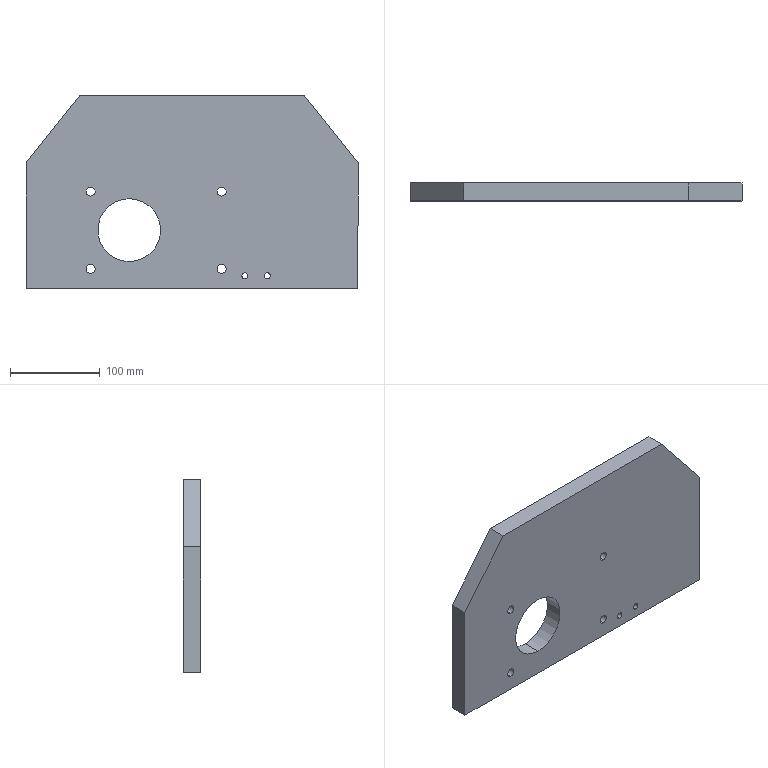Part | SolidWorks | features BaseBody 1 | 1 solid | 22 faces | box 370 x 20 x 215 mm | volume 1416295 mm3 | cylinder 14 | plane 8 | commonest cylinder face diameters 10 x8 6.8 x4 70 x2
STEP:
#1=CARTESIAN_POINT('',(-70.,0.,30.));
#2=VERTEX_POINT('',#1);
#3=CARTESIAN_POINT('',(-70.,0.,100.));
#4=VERTEX_POINT('',#3);
#5=CARTESIAN_POINT('',(-70.,0.,65.));
#6=DIRECTION('',(0.,1.,0.));
#7=DIRECTION('',(0.,0.,1.));
#8=AXIS2_PLACEMENT_3D('',#5,#6,#7);
#9=CIRCLE('',#8,35.);
#10=EDGE_CURVE('',#2,#4,#9,.T.);
#11=ORIENTED_EDGE('',*,*,#10,.F.);
#12=CARTESIAN_POINT('',(-70.,20.,30.));
#13=VERTEX_POINT('',#12);
#14=CARTESIAN_POINT('',(-70.,0.,30.));
#15=DIRECTION('',(0.,1.,0.));
#16=VECTOR('',#15,1000.);
#17=LINE('',#14,#16);
#18=EDGE_CURVE('',#2,#13,#17,.T.);
#19=ORIENTED_EDGE('',*,*,#18,.T.);
#20=CARTESIAN_POINT('',(-70.,20.,100.));
#21=VERTEX_POINT('',#20);
#22=CARTESIAN_POINT('',(-70.,20.,65.));
#23=DIRECTION('',(0.,-1.,0.));
#24=DIRECTION('',(0.,0.,1.));
#25=AXIS2_PLACEMENT_3D('',#22,#23,#24);
#26=CIRCLE('',#25,35.);
#27=EDGE_CURVE('',#21,#13,#26,.T.);
#28=ORIENTED_EDGE('',*,*,#27,.F.);
#29=CARTESIAN_POINT('',(-70.,0.,100.));
#30=DIRECTION('',(0.,1.,0.));
#31=VECTOR('',#30,1000.);
#32=LINE('',#29,#31);
#33=EDGE_CURVE('',#4,#21,#32,.T.);
#34=ORIENTED_EDGE('',*,*,#33,.F.);
#35=EDGE_LOOP('',(#11,#19,#28,#34));
#36=FACE_OUTER_BOUND('',#35,.T.);
#37=CARTESIAN_POINT('',(-70.,0.,65.));
#38=DIRECTION('',(0.,1.,0.));
#39=DIRECTION('',(0.,0.,1.));
#40=AXIS2_PLACEMENT_3D('',#37,#38,#39);
#41=CYLINDRICAL_SURFACE('',#40,35.);
#42=ADVANCED_FACE('',(#36),#41,.F.);
#43=CARTESIAN_POINT('',(-113.,0.,17.));
#44=VERTEX_POINT('',#43);
#45=CARTESIAN_POINT('',(-113.,0.,27.));
#46=VERTEX_POINT('',#45);
#47=CARTESIAN_POINT('',(-113.,0.,22.));
#48=DIRECTION('',(0.,1.,0.));
#49=DIRECTION('',(0.,0.,1.));
#50=AXIS2_PLACEMENT_3D('',#47,#48,#49);
#51=CIRCLE('',#50,5.);
#52=EDGE_CURVE('',#44,#46,#51,.T.);
#53=ORIENTED_EDGE('',*,*,#52,.F.);
#54=CARTESIAN_POINT('',(-113.,20.,17.));
#55=VERTEX_POINT('',#54);
#56=CARTESIAN_POINT('',(-113.,0.,17.));
#57=DIRECTION('',(0.,1.,0.));
#58=VECTOR('',#57,1000.);
#59=LINE('',#56,#58);
#60=EDGE_CURVE('',#44,#55,#59,.T.);
#61=ORIENTED_EDGE('',*,*,#60,.T.);
#62=CARTESIAN_POINT('',(-113.,20.,27.));
#63=VERTEX_POINT('',#62);
#64=CARTESIAN_POINT('',(-113.,20.,22.));
#65=DIRECTION('',(0.,-1.,0.));
#66=DIRECTION('',(0.,0.,1.));
#67=AXIS2_PLACEMENT_3D('',#64,#65,#66);
#68=CIRCLE('',#67,5.);
#69=EDGE_CURVE('',#63,#55,#68,.T.);
#70=ORIENTED_EDGE('',*,*,#69,.F.);
#71=CARTESIAN_POINT('',(-113.,0.,27.));
#72=DIRECTION('',(0.,1.,0.));
#73=VECTOR('',#72,1000.);
#74=LINE('',#71,#73);
#75=EDGE_CURVE('',#46,#63,#74,.T.);
#76=ORIENTED_EDGE('',*,*,#75,.F.);
#77=EDGE_LOOP('',(#53,#61,#70,#76));
#78=FACE_OUTER_BOUND('',#77,.T.);
#79=CARTESIAN_POINT('',(-113.,0.,22.));
#80=DIRECTION('',(0.,1.,0.));
#81=DIRECTION('',(0.,0.,1.));
#82=AXIS2_PLACEMENT_3D('',#79,#80,#81);
#83=CYLINDRICAL_SURFACE('',#82,5.);
#84=ADVANCED_FACE('',(#78),#83,.F.);
#85=CARTESIAN_POINT('',(33.,0.,17.));
#86=VERTEX_POINT('',#85);
#87=CARTESIAN_POINT('',(33.,0.,27.));
#88=VERTEX_POINT('',#87);
#89=CARTESIAN_POINT('',(33.,0.,22.));
#90=DIRECTION('',(0.,1.,0.));
#91=DIRECTION('',(0.,0.,1.));
#92=AXIS2_PLACEMENT_3D('',#89,#90,#91);
#93=CIRCLE('',#92,5.);
#94=EDGE_CURVE('',#86,#88,#93,.T.);
#95=ORIENTED_EDGE('',*,*,#94,.F.);
#96=CARTESIAN_POINT('',(33.,20.,17.));
#97=VERTEX_POINT('',#96);
#98=CARTESIAN_POINT('',(33.,0.,17.));
#99=DIRECTION('',(0.,1.,0.));
#100=VECTOR('',#99,1000.);
#101=LINE('',#98,#100);
#102=EDGE_CURVE('',#86,#97,#101,.T.);
#103=ORIENTED_EDGE('',*,*,#102,.T.);
#104=CARTESIAN_POINT('',(33.,20.,27.));
#105=VERTEX_POINT('',#104);
#106=CARTESIAN_POINT('',(33.,20.,22.));
#107=DIRECTION('',(0.,-1.,0.));
#108=DIRECTION('',(0.,0.,1.));
#109=AXIS2_PLACEMENT_3D('',#106,#107,#108);
#110=CIRCLE('',#109,5.);
#111=EDGE_CURVE('',#105,#97,#110,.T.);
#112=ORIENTED_EDGE('',*,*,#111,.F.);
#113=CARTESIAN_POINT('',(33.,0.,27.));
#114=DIRECTION('',(0.,1.,0.));
#115=VECTOR('',#114,1000.);
#116=LINE('',#113,#115);
#117=EDGE_CURVE('',#88,#105,#116,.T.);
#118=ORIENTED_EDGE('',*,*,#117,.F.);
#119=EDGE_LOOP('',(#95,#103,#112,#118));
#120=FACE_OUTER_BOUND('',#119,.T.);
#121=CARTESIAN_POINT('',(33.,0.,22.));
#122=DIRECTION('',(0.,1.,0.));
#123=DIRECTION('',(0.,0.,1.));
#124=AXIS2_PLACEMENT_3D('',#121,#122,#123);
#125=CYLINDRICAL_SURFACE('',#124,5.);
#126=ADVANCED_FACE('',(#120),#125,.F.);
#127=CARTESIAN_POINT('',(33.,0.,103.));
#128=VERTEX_POINT('',#127);
#129=CARTESIAN_POINT('',(33.,0.,113.));
#130=VERTEX_POINT('',#129);
#131=CARTESIAN_POINT('',(33.,0.,108.));
#132=DIRECTION('',(0.,1.,0.));
#133=DIRECTION('',(0.,0.,1.));
#134=AXIS2_PLACEMENT_3D('',#131,#132,#133);
#135=CIRCLE('',#134,5.);
#136=EDGE_CURVE('',#128,#130,#135,.T.);
#137=ORIENTED_EDGE('',*,*,#136,.F.);
#138=CARTESIAN_POINT('',(33.,20.,103.));
#139=VERTEX_POINT('',#138);
#140=CARTESIAN_POINT('',(33.,0.,103.));
#141=DIRECTION('',(0.,1.,0.));
#142=VECTOR('',#141,1000.);
#143=LINE('',#140,#142);
#144=EDGE_CURVE('',#128,#139,#143,.T.);
#145=ORIENTED_EDGE('',*,*,#144,.T.);
#146=CARTESIAN_POINT('',(33.,20.,113.));
#147=VERTEX_POINT('',#146);
#148=CARTESIAN_POINT('',(33.,20.,108.));
#149=DIRECTION('',(0.,-1.,0.));
#150=DIRECTION('',(0.,0.,1.));
#151=AXIS2_PLACEMENT_3D('',#148,#149,#150);
#152=CIRCLE('',#151,5.);
#153=EDGE_CURVE('',#147,#139,#152,.T.);
#154=ORIENTED_EDGE('',*,*,#153,.F.);
#155=CARTESIAN_POINT('',(33.,0.,113.));
#156=DIRECTION('',(0.,1.,0.));
#157=VECTOR('',#156,1000.);
#158=LINE('',#155,#157);
#159=EDGE_CURVE('',#130,#147,#158,.T.);
#160=ORIENTED_EDGE('',*,*,#159,.F.);
#161=EDGE_LOOP('',(#137,#145,#154,#160));
#162=FACE_OUTER_BOUND('',#161,.T.);
#163=CARTESIAN_POINT('',(33.,0.,108.));
#164=DIRECTION('',(0.,1.,0.));
#165=DIRECTION('',(0.,0.,1.));
#166=AXIS2_PLACEMENT_3D('',#163,#164,#165);
#167=CYLINDRICAL_SURFACE('',#166,5.);
#168=ADVANCED_FACE('',(#162),#167,.F.);
#169=CARTESIAN_POINT('',(-113.,0.,103.));
#170=VERTEX_POINT('',#169);
#171=CARTESIAN_POINT('',(-113.,0.,113.));
#172=VERTEX_POINT('',#171);
#173=CARTESIAN_POINT('',(-113.,0.,108.));
#174=DIRECTION('',(0.,1.,0.));
#175=DIRECTION('',(0.,0.,1.));
#176=AXIS2_PLACEMENT_3D('',#173,#174,#175);
#177=CIRCLE('',#176,5.);
#178=EDGE_CURVE('',#170,#172,#177,.T.);
#179=ORIENTED_EDGE('',*,*,#178,.F.);
#180=CARTESIAN_POINT('',(-113.,20.,103.));
#181=VERTEX_POINT('',#180);
#182=CARTESIAN_POINT('',(-113.,0.,103.));
#183=DIRECTION('',(0.,1.,0.));
#184=VECTOR('',#183,1000.);
#185=LINE('',#182,#184);
#186=EDGE_CURVE('',#170,#181,#185,.T.);
#187=ORIENTED_EDGE('',*,*,#186,.T.);
#188=CARTESIAN_POINT('',(-113.,20.,113.));
#189=VERTEX_POINT('',#188);
#190=CARTESIAN_POINT('',(-113.,20.,108.));
#191=DIRECTION('',(0.,-1.,0.));
#192=DIRECTION('',(0.,0.,1.));
#193=AXIS2_PLACEMENT_3D('',#190,#191,#192);
#194=CIRCLE('',#193,5.);
#195=EDGE_CURVE('',#189,#181,#194,.T.);
#196=ORIENTED_EDGE('',*,*,#195,.F.);
#197=CARTESIAN_POINT('',(-113.,0.,113.));
#198=DIRECTION('',(0.,1.,0.));
#199=VECTOR('',#198,1000.);
#200=LINE('',#197,#199);
#201=EDGE_CURVE('',#172,#189,#200,.T.);
#202=ORIENTED_EDGE('',*,*,#201,.F.);
#203=EDGE_LOOP('',(#179,#187,#196,#202));
#204=FACE_OUTER_BOUND('',#203,.T.);
#205=CARTESIAN_POINT('',(-113.,0.,108.));
#206=DIRECTION('',(0.,1.,0.));
#207=DIRECTION('',(0.,0.,1.));
#208=AXIS2_PLACEMENT_3D('',#205,#206,#207);
#209=CYLINDRICAL_SURFACE('',#208,5.);
#210=ADVANCED_FACE('',(#204),#209,.F.);
#211=CARTESIAN_POINT('',(83.921,20.,17.4));
#212=VERTEX_POINT('',#211);
#213=CARTESIAN_POINT('',(83.921,20.,10.6));
#214=VERTEX_POINT('',#213);
#215=CARTESIAN_POINT('',(83.921,20.,14.));
#216=DIRECTION('',(0.,-1.,0.));
#217=DIRECTION('',(0.,0.,-1.));
#218=AXIS2_PLACEMENT_3D('',#215,#216,#217);
#219=CIRCLE('',#218,3.4);
#220=EDGE_CURVE('',#212,#214,#219,.T.);
#221=ORIENTED_EDGE('',*,*,#220,.F.);
#222=CARTESIAN_POINT('',(83.921,0.,17.4));
#223=VERTEX_POINT('',#222);
#224=CARTESIAN_POINT('',(83.921,0.,17.4));
#225=DIRECTION('',(0.,-1.,0.));
#226=VECTOR('',#225,1000.);
#227=LINE('',#224,#226);
#228=EDGE_CURVE('',#212,#223,#227,.T.);
#229=ORIENTED_EDGE('',*,*,#228,.T.);
#230=CARTESIAN_POINT('',(83.921,0.,10.6));
#231=VERTEX_POINT('',#230);
#232=CARTESIAN_POINT('',(83.921,0.,14.));
#233=DIRECTION('',(0.,1.,0.));
#234=DIRECTION('',(0.,0.,-1.));
#235=AXIS2_PLACEMENT_3D('',#232,#233,#234);
#236=CIRCLE('',#235,3.4);
#237=EDGE_CURVE('',#231,#223,#236,.T.);
#238=ORIENTED_EDGE('',*,*,#237,.F.);
#239=CARTESIAN_POINT('',(83.921,0.,10.6));
#240=DIRECTION('',(0.,-1.,0.));
#241=VECTOR('',#240,1000.);
#242=LINE('',#239,#241);
#243=EDGE_CURVE('',#214,#231,#242,.T.);
#244=ORIENTED_EDGE('',*,*,#243,.F.);
#245=EDGE_LOOP('',(#221,#229,#238,#244));
#246=FACE_OUTER_BOUND('',#245,.T.);
#247=CARTESIAN_POINT('',(83.921,0.,14.));
#248=DIRECTION('',(0.,-1.,0.));
#249=DIRECTION('',(0.,0.,-1.));
#250=AXIS2_PLACEMENT_3D('',#247,#248,#249);
#251=CYLINDRICAL_SURFACE('',#250,3.4);
#252=ADVANCED_FACE('',(#246),#251,.F.);
#253=CARTESIAN_POINT('',(58.921,20.,17.4));
#254=VERTEX_POINT('',#253);
#255=CARTESIAN_POINT('',(58.921,20.,10.6));
#256=VERTEX_POINT('',#255);
#257=CARTESIAN_POINT('',(58.921,20.,14.));
#258=DIRECTION('',(0.,-1.,0.));
#259=DIRECTION('',(0.,0.,-1.));
#260=AXIS2_PLACEMENT_3D('',#257,#258,#259);
#261=CIRCLE('',#260,3.4);
#262=EDGE_CURVE('',#254,#256,#261,.T.);
#263=ORIENTED_EDGE('',*,*,#262,.F.);
#264=CARTESIAN_POINT('',(58.921,0.,17.4));
#265=VERTEX_POINT('',#264);
#266=CARTESIAN_POINT('',(58.921,0.,17.4));
#267=DIRECTION('',(0.,-1.,0.));
#268=VECTOR('',#267,1000.);
#269=LINE('',#266,#268);
#270=EDGE_CURVE('',#254,#265,#269,.T.);
#271=ORIENTED_EDGE('',*,*,#270,.T.);
#272=CARTESIAN_POINT('',(58.921,0.,10.6));
#273=VERTEX_POINT('',#272);
#274=CARTESIAN_POINT('',(58.921,0.,14.));
#275=DIRECTION('',(0.,1.,0.));
#276=DIRECTION('',(0.,0.,-1.));
#277=AXIS2_PLACEMENT_3D('',#274,#275,#276);
#278=CIRCLE('',#277,3.4);
#279=EDGE_CURVE('',#273,#265,#278,.T.);
#280=ORIENTED_EDGE('',*,*,#279,.F.);
#281=CARTESIAN_POINT('',(58.921,0.,10.6));
#282=DIRECTION('',(0.,-1.,0.));
#283=VECTOR('',#282,1000.);
#284=LINE('',#281,#283);
#285=EDGE_CURVE('',#256,#273,#284,.T.);
#286=ORIENTED_EDGE('',*,*,#285,.F.);
#287=EDGE_LOOP('',(#263,#271,#280,#286));
#288=FACE_OUTER_BOUND('',#287,.T.);
#289=CARTESIAN_POINT('',(58.921,0.,14.));
#290=DIRECTION('',(0.,-1.,0.));
#291=DIRECTION('',(0.,0.,-1.));
#292=AXIS2_PLACEMENT_3D('',#289,#290,#291);
#293=CYLINDRICAL_SURFACE('',#292,3.4);
#294=ADVANCED_FACE('',(#288),#293,.F.);
#295=CARTESIAN_POINT('',(185.,20.,140.));
#296=VERTEX_POINT('',#295);
#297=CARTESIAN_POINT('',(185.,20.,0.));
#298=VERTEX_POINT('',#297);
#299=CARTESIAN_POINT('',(185.,20.,0.));
#300=DIRECTION('',(0.,0.,-1.));
#301=VECTOR('',#300,1000.);
#302=LINE('',#299,#301);
#303=EDGE_CURVE('',#296,#298,#302,.T.);
#304=ORIENTED_EDGE('',*,*,#303,.T.);
#305=CARTESIAN_POINT('',(-185.,20.,0.));
#306=VERTEX_POINT('',#305);
#307=CARTESIAN_POINT('',(0.,20.,0.));
#308=DIRECTION('',(-1.,0.,0.));
#309=VECTOR('',#308,1000.);
#310=LINE('',#307,#309);
#311=EDGE_CURVE('',#298,#306,#310,.T.);
#312=ORIENTED_EDGE('',*,*,#311,.T.);
#313=CARTESIAN_POINT('',(-185.,20.,140.));
#314=VERTEX_POINT('',#313);
#315=CARTESIAN_POINT('',(-185.,20.,0.));
#316=DIRECTION('',(0.,0.,1.));
#317=VECTOR('',#316,1000.);
#318=LINE('',#315,#317);
#319=EDGE_CURVE('',#306,#314,#318,.T.);
#320=ORIENTED_EDGE('',*,*,#319,.T.);
#321=CARTESIAN_POINT('',(-125.,20.,215.));
#322=VERTEX_POINT('',#321);
#323=CARTESIAN_POINT('',(-185.,20.,140.));
#324=DIRECTION('',(0.6247,0.,0.7809));
#325=VECTOR('',#324,1000.);
#326=LINE('',#323,#325);
#327=EDGE_CURVE('',#314,#322,#326,.T.);
#328=ORIENTED_EDGE('',*,*,#327,.T.);
#329=CARTESIAN_POINT('',(125.,20.,215.));
#330=VERTEX_POINT('',#329);
#331=CARTESIAN_POINT('',(0.,20.,215.));
#332=DIRECTION('',(1.,0.,0.));
#333=VECTOR('',#332,1000.);
#334=LINE('',#331,#333);
#335=EDGE_CURVE('',#322,#330,#334,.T.);
#336=ORIENTED_EDGE('',*,*,#335,.T.);
#337=CARTESIAN_POINT('',(125.,20.,215.));
#338=DIRECTION('',(0.6247,0.,-0.7809));
#339=VECTOR('',#338,1000.);
#340=LINE('',#337,#339);
#341=EDGE_CURVE('',#330,#296,#340,.T.);
#342=ORIENTED_EDGE('',*,*,#341,.T.);
#343=EDGE_LOOP('',(#304,#312,#320,#328,#336,#342));
#344=FACE_OUTER_BOUND('',#343,.T.);
#345=ORIENTED_EDGE('',*,*,#27,.T.);
#346=CARTESIAN_POINT('',(-70.,20.,65.));
#347=DIRECTION('',(0.,-1.,0.));
#348=DIRECTION('',(0.,0.,1.));
#349=AXIS2_PLACEMENT_3D('',#346,#347,#348);
#350=CIRCLE('',#349,35.);
#351=EDGE_CURVE('',#13,#21,#350,.T.);
#352=ORIENTED_EDGE('',*,*,#351,.T.);
#353=EDGE_LOOP('',(#345,#352));
#354=FACE_BOUND('',#353,.T.);
#355=ORIENTED_EDGE('',*,*,#69,.T.);
#356=CARTESIAN_POINT('',(-113.,20.,22.));
#357=DIRECTION('',(0.,-1.,0.));
#358=DIRECTION('',(0.,0.,1.));
#359=AXIS2_PLACEMENT_3D('',#356,#357,#358);
#360=CIRCLE('',#359,5.);
#361=EDGE_CURVE('',#55,#63,#360,.T.);
#362=ORIENTED_EDGE('',*,*,#361,.T.);
#363=EDGE_LOOP('',(#355,#362));
#364=FACE_BOUND('',#363,.T.);
#365=ORIENTED_EDGE('',*,*,#111,.T.);
#366=CARTESIAN_POINT('',(33.,20.,22.));
#367=DIRECTION('',(0.,-1.,0.));
#368=DIRECTION('',(0.,0.,1.));
#369=AXIS2_PLACEMENT_3D('',#366,#367,#368);
#370=CIRCLE('',#369,5.);
#371=EDGE_CURVE('',#97,#105,#370,.T.);
#372=ORIENTED_EDGE('',*,*,#371,.T.);
#373=EDGE_LOOP('',(#365,#372));
#374=FACE_BOUND('',#373,.T.);
#375=ORIENTED_EDGE('',*,*,#153,.T.);
#376=CARTESIAN_POINT('',(33.,20.,108.));
#377=DIRECTION('',(0.,-1.,0.));
#378=DIRECTION('',(0.,0.,1.));
#379=AXIS2_PLACEMENT_3D('',#376,#377,#378);
#380=CIRCLE('',#379,5.);
#381=EDGE_CURVE('',#139,#147,#380,.T.);
#382=ORIENTED_EDGE('',*,*,#381,.T.);
#383=EDGE_LOOP('',(#375,#382));
#384=FACE_BOUND('',#383,.T.);
#385=ORIENTED_EDGE('',*,*,#195,.T.);
#386=CARTESIAN_POINT('',(-113.,20.,108.));
#387=DIRECTION('',(0.,-1.,0.));
#388=DIRECTION('',(0.,0.,1.));
#389=AXIS2_PLACEMENT_3D('',#386,#387,#388);
#390=CIRCLE('',#389,5.);
#391=EDGE_CURVE('',#181,#189,#390,.T.);
#392=ORIENTED_EDGE('',*,*,#391,.T.);
#393=EDGE_LOOP('',(#385,#392));
#394=FACE_BOUND('',#393,.T.);
#395=CARTESIAN_POINT('',(83.921,20.,14.));
#396=DIRECTION('',(0.,-1.,0.));
#397=DIRECTION('',(0.,0.,-1.));
#398=AXIS2_PLACEMENT_3D('',#395,#396,#397);
#399=CIRCLE('',#398,3.4);
#400=EDGE_CURVE('',#214,#212,#399,.T.);
#401=ORIENTED_EDGE('',*,*,#400,.T.);
#402=ORIENTED_EDGE('',*,*,#220,.T.);
#403=EDGE_LOOP('',(#401,#402));
#404=FACE_BOUND('',#403,.T.);
#405=CARTESIAN_POINT('',(58.921,20.,14.));
#406=DIRECTION('',(0.,-1.,0.));
#407=DIRECTION('',(0.,0.,-1.));
#408=AXIS2_PLACEMENT_3D('',#405,#406,#407);
#409=CIRCLE('',#408,3.4);
#410=EDGE_CURVE('',#256,#254,#409,.T.);
#411=ORIENTED_EDGE('',*,*,#410,.T.);
#412=ORIENTED_EDGE('',*,*,#262,.T.);
#413=EDGE_LOOP('',(#411,#412));
#414=FACE_BOUND('',#413,.T.);
#415=CARTESIAN_POINT('',(0.,20.,0.));
#416=DIRECTION('',(0.,1.,0.));
#417=DIRECTION('',(0.,0.,1.));
#418=AXIS2_PLACEMENT_3D('',#415,#416,#417);
#419=PLANE('',#418);
#420=ADVANCED_FACE('',(#344,#354,#364,#374,#384,#394,#404,#414),#419,.T.);
#421=CARTESIAN_POINT('',(-185.,0.,0.));
#422=VERTEX_POINT('',#421);
#423=CARTESIAN_POINT('',(-185.,20.,0.));
#424=DIRECTION('',(0.,-1.,0.));
#425=VECTOR('',#424,1000.);
#426=LINE('',#423,#425);
#427=EDGE_CURVE('',#306,#422,#426,.T.);
#428=ORIENTED_EDGE('',*,*,#427,.F.);
#429=ORIENTED_EDGE('',*,*,#311,.F.);
#430=CARTESIAN_POINT('',(185.,0.,0.));
#431=VERTEX_POINT('',#430);
#432=CARTESIAN_POINT('',(185.,20.,0.));
#433=DIRECTION('',(0.,1.,0.));
#434=VECTOR('',#433,1000.);
#435=LINE('',#432,#434);
#436=EDGE_CURVE('',#431,#298,#435,.T.);
#437=ORIENTED_EDGE('',*,*,#436,.F.);
#438=CARTESIAN_POINT('',(-185.,0.,0.));
#439=DIRECTION('',(1.,0.,0.));
#440=VECTOR('',#439,1000.);
#441=LINE('',#438,#440);
#442=EDGE_CURVE('',#422,#431,#441,.T.);
#443=ORIENTED_EDGE('',*,*,#442,.F.);
#444=EDGE_LOOP('',(#428,#429,#437,#443));
#445=FACE_OUTER_BOUND('',#444,.T.);
#446=CARTESIAN_POINT('',(-185.,20.,0.));
#447=DIRECTION('',(0.,0.,1.));
#448=DIRECTION('',(1.,0.,0.));
#449=AXIS2_PLACEMENT_3D('',#446,#447,#448);
#450=PLANE('',#449);
#451=ADVANCED_FACE('',(#445),#450,.F.);
#452=ORIENTED_EDGE('',*,*,#436,.T.);
#453=ORIENTED_EDGE('',*,*,#303,.F.);
#454=CARTESIAN_POINT('',(185.,0.,140.));
#455=VERTEX_POINT('',#454);
#456=CARTESIAN_POINT('',(185.,20.,140.));
#457=DIRECTION('',(0.,1.,0.));
#458=VECTOR('',#457,1000.);
#459=LINE('',#456,#458);
#460=EDGE_CURVE('',#455,#296,#459,.T.);
#461=ORIENTED_EDGE('',*,*,#460,.F.);
#462=CARTESIAN_POINT('',(185.,0.,0.));
#463=DIRECTION('',(0.,0.,1.));
#464=VECTOR('',#463,1000.);
#465=LINE('',#462,#464);
#466=EDGE_CURVE('',#431,#455,#465,.T.);
#467=ORIENTED_EDGE('',*,*,#466,.F.);
#468=EDGE_LOOP('',(#452,#453,#461,#467));
#469=FACE_OUTER_BOUND('',#468,.T.);
#470=CARTESIAN_POINT('',(185.,20.,0.));
#471=DIRECTION('',(-1.,0.,0.));
#472=DIRECTION('',(0.,0.,1.));
#473=AXIS2_PLACEMENT_3D('',#470,#471,#472);
#474=PLANE('',#473);
#475=ADVANCED_FACE('',(#469),#474,.F.);
#476=ORIENTED_EDGE('',*,*,#460,.T.);
#477=ORIENTED_EDGE('',*,*,#341,.F.);
#478=CARTESIAN_POINT('',(125.,0.,215.));
#479=VERTEX_POINT('',#478);
#480=CARTESIAN_POINT('',(125.,20.,215.));
#481=DIRECTION('',(0.,1.,0.));
#482=VECTOR('',#481,1000.);
#483=LINE('',#480,#482);
#484=EDGE_CURVE('',#479,#330,#483,.T.);
#485=ORIENTED_EDGE('',*,*,#484,.F.);
#486=CARTESIAN_POINT('',(185.,0.,140.));
#487=DIRECTION('',(-0.6247,0.,0.7809));
#488=VECTOR('',#487,1000.);
#489=LINE('',#486,#488);
#490=EDGE_CURVE('',#455,#479,#489,.T.);
#491=ORIENTED_EDGE('',*,*,#490,.F.);
#492=EDGE_LOOP('',(#476,#477,#485,#491));
#493=FACE_OUTER_BOUND('',#492,.T.);
#494=CARTESIAN_POINT('',(185.,20.,140.));
#495=DIRECTION('',(-0.7809,0.,-0.6247));
#496=DIRECTION('',(-0.6247,0.,0.7809));
#497=AXIS2_PLACEMENT_3D('',#494,#495,#496);
#498=PLANE('',#497);
#499=ADVANCED_FACE('',(#493),#498,.F.);
#500=ORIENTED_EDGE('',*,*,#484,.T.);
#501=ORIENTED_EDGE('',*,*,#335,.F.);
#502=CARTESIAN_POINT('',(-125.,0.,215.));
#503=VERTEX_POINT('',#502);
#504=CARTESIAN_POINT('',(-125.,20.,215.));
#505=DIRECTION('',(0.,1.,0.));
#506=VECTOR('',#505,1000.);
#507=LINE('',#504,#506);
#508=EDGE_CURVE('',#503,#322,#507,.T.);
#509=ORIENTED_EDGE('',*,*,#508,.F.);
#510=CARTESIAN_POINT('',(-125.,0.,215.));
#511=DIRECTION('',(-1.,0.,0.));
#512=VECTOR('',#511,1000.);
#513=LINE('',#510,#512);
#514=EDGE_CURVE('',#479,#503,#513,.T.);
#515=ORIENTED_EDGE('',*,*,#514,.F.);
#516=EDGE_LOOP('',(#500,#501,#509,#515));
#517=FACE_OUTER_BOUND('',#516,.T.);
#518=CARTESIAN_POINT('',(-125.,20.,215.));
#519=DIRECTION('',(0.,0.,-1.));
#520=DIRECTION('',(-1.,0.,0.));
#521=AXIS2_PLACEMENT_3D('',#518,#519,#520);
#522=PLANE('',#521);
#523=ADVANCED_FACE('',(#517),#522,.F.);
#524=ORIENTED_EDGE('',*,*,#508,.T.);
#525=ORIENTED_EDGE('',*,*,#327,.F.);
#526=CARTESIAN_POINT('',(-185.,0.,140.));
#527=VERTEX_POINT('',#526);
#528=CARTESIAN_POINT('',(-185.,20.,140.));
#529=DIRECTION('',(0.,1.,0.));
#530=VECTOR('',#529,1000.);
#531=LINE('',#528,#530);
#532=EDGE_CURVE('',#527,#314,#531,.T.);
#533=ORIENTED_EDGE('',*,*,#532,.F.);
#534=CARTESIAN_POINT('',(-185.,0.,140.));
#535=DIRECTION('',(-0.6247,0.,-0.7809));
#536=VECTOR('',#535,1000.);
#537=LINE('',#534,#536);
#538=EDGE_CURVE('',#503,#527,#537,.T.);
#539=ORIENTED_EDGE('',*,*,#538,.F.);
#540=EDGE_LOOP('',(#524,#525,#533,#539));
#541=FACE_OUTER_BOUND('',#540,.T.);
#542=CARTESIAN_POINT('',(-185.,20.,140.));
#543=DIRECTION('',(0.7809,0.,-0.6247));
#544=DIRECTION('',(-0.6247,0.,-0.7809));
#545=AXIS2_PLACEMENT_3D('',#542,#543,#544);
#546=PLANE('',#545);
#547=ADVANCED_FACE('',(#541),#546,.F.);
#548=ORIENTED_EDGE('',*,*,#532,.T.);
#549=ORIENTED_EDGE('',*,*,#319,.F.);
#550=ORIENTED_EDGE('',*,*,#427,.T.);
#551=CARTESIAN_POINT('',(-185.,0.,0.));
#552=DIRECTION('',(0.,0.,-1.));
#553=VECTOR('',#552,1000.);
#554=LINE('',#551,#553);
#555=EDGE_CURVE('',#527,#422,#554,.T.);
#556=ORIENTED_EDGE('',*,*,#555,.F.);
#557=EDGE_LOOP('',(#548,#549,#550,#556));
#558=FACE_OUTER_BOUND('',#557,.T.);
#559=CARTESIAN_POINT('',(-185.,20.,0.));
#560=DIRECTION('',(1.,0.,0.));
#561=DIRECTION('',(0.,0.,-1.));
#562=AXIS2_PLACEMENT_3D('',#559,#560,#561);
#563=PLANE('',#562);
#564=ADVANCED_FACE('',(#558),#563,.F.);
#565=ORIENTED_EDGE('',*,*,#18,.F.);
#566=CARTESIAN_POINT('',(-70.,0.,65.));
#567=DIRECTION('',(0.,1.,0.));
#568=DIRECTION('',(0.,0.,1.));
#569=AXIS2_PLACEMENT_3D('',#566,#567,#568);
#570=CIRCLE('',#569,35.);
#571=EDGE_CURVE('',#4,#2,#570,.T.);
#572=ORIENTED_EDGE('',*,*,#571,.F.);
#573=ORIENTED_EDGE('',*,*,#33,.T.);
#574=ORIENTED_EDGE('',*,*,#351,.F.);
#575=EDGE_LOOP('',(#565,#572,#573,#574));
#576=FACE_OUTER_BOUND('',#575,.T.);
#577=CARTESIAN_POINT('',(-70.,0.,65.));
#578=DIRECTION('',(0.,1.,0.));
#579=DIRECTION('',(0.,0.,1.));
#580=AXIS2_PLACEMENT_3D('',#577,#578,#579);
#581=CYLINDRICAL_SURFACE('',#580,35.);
#582=ADVANCED_FACE('',(#576),#581,.F.);
#583=ORIENTED_EDGE('',*,*,#60,.F.);
#584=CARTESIAN_POINT('',(-113.,0.,22.));
#585=DIRECTION('',(0.,1.,0.));
#586=DIRECTION('',(0.,0.,1.));
#587=AXIS2_PLACEMENT_3D('',#584,#585,#586);
#588=CIRCLE('',#587,5.);
#589=EDGE_CURVE('',#46,#44,#588,.T.);
#590=ORIENTED_EDGE('',*,*,#589,.F.);
#591=ORIENTED_EDGE('',*,*,#75,.T.);
#592=ORIENTED_EDGE('',*,*,#361,.F.);
#593=EDGE_LOOP('',(#583,#590,#591,#592));
#594=FACE_OUTER_BOUND('',#593,.T.);
#595=CARTESIAN_POINT('',(-113.,0.,22.));
#596=DIRECTION('',(0.,1.,0.));
#597=DIRECTION('',(0.,0.,1.));
#598=AXIS2_PLACEMENT_3D('',#595,#596,#597);
#599=CYLINDRICAL_SURFACE('',#598,5.);
#600=ADVANCED_FACE('',(#594),#599,.F.);
#601=ORIENTED_EDGE('',*,*,#102,.F.);
#602=CARTESIAN_POINT('',(33.,0.,22.));
#603=DIRECTION('',(0.,1.,0.));
#604=DIRECTION('',(0.,0.,1.));
#605=AXIS2_PLACEMENT_3D('',#602,#603,#604);
#606=CIRCLE('',#605,5.);
#607=EDGE_CURVE('',#88,#86,#606,.T.);
#608=ORIENTED_EDGE('',*,*,#607,.F.);
#609=ORIENTED_EDGE('',*,*,#117,.T.);
#610=ORIENTED_EDGE('',*,*,#371,.F.);
#611=EDGE_LOOP('',(#601,#608,#609,#610));
#612=FACE_OUTER_BOUND('',#611,.T.);
#613=CARTESIAN_POINT('',(33.,0.,22.));
#614=DIRECTION('',(0.,1.,0.));
#615=DIRECTION('',(0.,0.,1.));
#616=AXIS2_PLACEMENT_3D('',#613,#614,#615);
#617=CYLINDRICAL_SURFACE('',#616,5.);
#618=ADVANCED_FACE('',(#612),#617,.F.);
#619=ORIENTED_EDGE('',*,*,#144,.F.);
#620=CARTESIAN_POINT('',(33.,0.,108.));
#621=DIRECTION('',(0.,1.,0.));
#622=DIRECTION('',(0.,0.,1.));
#623=AXIS2_PLACEMENT_3D('',#620,#621,#622);
#624=CIRCLE('',#623,5.);
#625=EDGE_CURVE('',#130,#128,#624,.T.);
#626=ORIENTED_EDGE('',*,*,#625,.F.);
#627=ORIENTED_EDGE('',*,*,#159,.T.);
#628=ORIENTED_EDGE('',*,*,#381,.F.);
#629=EDGE_LOOP('',(#619,#626,#627,#628));
#630=FACE_OUTER_BOUND('',#629,.T.);
#631=CARTESIAN_POINT('',(33.,0.,108.));
#632=DIRECTION('',(0.,1.,0.));
#633=DIRECTION('',(0.,0.,1.));
#634=AXIS2_PLACEMENT_3D('',#631,#632,#633);
#635=CYLINDRICAL_SURFACE('',#634,5.);
#636=ADVANCED_FACE('',(#630),#635,.F.);
#637=ORIENTED_EDGE('',*,*,#186,.F.);
#638=CARTESIAN_POINT('',(-113.,0.,108.));
#639=DIRECTION('',(0.,1.,0.));
#640=DIRECTION('',(0.,0.,1.));
#641=AXIS2_PLACEMENT_3D('',#638,#639,#640);
#642=CIRCLE('',#641,5.);
#643=EDGE_CURVE('',#172,#170,#642,.T.);
#644=ORIENTED_EDGE('',*,*,#643,.F.);
#645=ORIENTED_EDGE('',*,*,#201,.T.);
#646=ORIENTED_EDGE('',*,*,#391,.F.);
#647=EDGE_LOOP('',(#637,#644,#645,#646));
#648=FACE_OUTER_BOUND('',#647,.T.);
#649=CARTESIAN_POINT('',(-113.,0.,108.));
#650=DIRECTION('',(0.,1.,0.));
#651=DIRECTION('',(0.,0.,1.));
#652=AXIS2_PLACEMENT_3D('',#649,#650,#651);
#653=CYLINDRICAL_SURFACE('',#652,5.);
#654=ADVANCED_FACE('',(#648),#653,.F.);
#655=ORIENTED_EDGE('',*,*,#228,.F.);
#656=ORIENTED_EDGE('',*,*,#400,.F.);
#657=ORIENTED_EDGE('',*,*,#243,.T.);
#658=CARTESIAN_POINT('',(83.921,0.,14.));
#659=DIRECTION('',(0.,1.,0.));
#660=DIRECTION('',(0.,0.,-1.));
#661=AXIS2_PLACEMENT_3D('',#658,#659,#660);
#662=CIRCLE('',#661,3.4);
#663=EDGE_CURVE('',#223,#231,#662,.T.);
#664=ORIENTED_EDGE('',*,*,#663,.F.);
#665=EDGE_LOOP('',(#655,#656,#657,#664));
#666=FACE_OUTER_BOUND('',#665,.T.);
#667=CARTESIAN_POINT('',(83.921,0.,14.));
#668=DIRECTION('',(0.,-1.,0.));
#669=DIRECTION('',(0.,0.,-1.));
#670=AXIS2_PLACEMENT_3D('',#667,#668,#669);
#671=CYLINDRICAL_SURFACE('',#670,3.4);
#672=ADVANCED_FACE('',(#666),#671,.F.);
#673=ORIENTED_EDGE('',*,*,#270,.F.);
#674=ORIENTED_EDGE('',*,*,#410,.F.);
#675=ORIENTED_EDGE('',*,*,#285,.T.);
#676=CARTESIAN_POINT('',(58.921,0.,14.));
#677=DIRECTION('',(0.,1.,0.));
#678=DIRECTION('',(0.,0.,-1.));
#679=AXIS2_PLACEMENT_3D('',#676,#677,#678);
#680=CIRCLE('',#679,3.4);
#681=EDGE_CURVE('',#265,#273,#680,.T.);
#682=ORIENTED_EDGE('',*,*,#681,.F.);
#683=EDGE_LOOP('',(#673,#674,#675,#682));
#684=FACE_OUTER_BOUND('',#683,.T.);
#685=CARTESIAN_POINT('',(58.921,0.,14.));
#686=DIRECTION('',(0.,-1.,0.));
#687=DIRECTION('',(0.,0.,-1.));
#688=AXIS2_PLACEMENT_3D('',#685,#686,#687);
#689=CYLINDRICAL_SURFACE('',#688,3.4);
#690=ADVANCED_FACE('',(#684),#689,.F.);
#691=ORIENTED_EDGE('',*,*,#442,.T.);
#692=ORIENTED_EDGE('',*,*,#466,.T.);
#693=ORIENTED_EDGE('',*,*,#490,.T.);
#694=ORIENTED_EDGE('',*,*,#514,.T.);
#695=ORIENTED_EDGE('',*,*,#538,.T.);
#696=ORIENTED_EDGE('',*,*,#555,.T.);
#697=EDGE_LOOP('',(#691,#692,#693,#694,#695,#696));
#698=FACE_OUTER_BOUND('',#697,.T.);
#699=ORIENTED_EDGE('',*,*,#571,.T.);
#700=ORIENTED_EDGE('',*,*,#10,.T.);
#701=EDGE_LOOP('',(#699,#700));
#702=FACE_BOUND('',#701,.T.);
#703=ORIENTED_EDGE('',*,*,#589,.T.);
#704=ORIENTED_EDGE('',*,*,#52,.T.);
#705=EDGE_LOOP('',(#703,#704));
#706=FACE_BOUND('',#705,.T.);
#707=ORIENTED_EDGE('',*,*,#607,.T.);
#708=ORIENTED_EDGE('',*,*,#94,.T.);
#709=EDGE_LOOP('',(#707,#708));
#710=FACE_BOUND('',#709,.T.);
#711=ORIENTED_EDGE('',*,*,#625,.T.);
#712=ORIENTED_EDGE('',*,*,#136,.T.);
#713=EDGE_LOOP('',(#711,#712));
#714=FACE_BOUND('',#713,.T.);
#715=ORIENTED_EDGE('',*,*,#643,.T.);
#716=ORIENTED_EDGE('',*,*,#178,.T.);
#717=EDGE_LOOP('',(#715,#716));
#718=FACE_BOUND('',#717,.T.);
#719=ORIENTED_EDGE('',*,*,#237,.T.);
#720=ORIENTED_EDGE('',*,*,#663,.T.);
#721=EDGE_LOOP('',(#719,#720));
#722=FACE_BOUND('',#721,.T.);
#723=ORIENTED_EDGE('',*,*,#279,.T.);
#724=ORIENTED_EDGE('',*,*,#681,.T.);
#725=EDGE_LOOP('',(#723,#724));
#726=FACE_BOUND('',#725,.T.);
#727=CARTESIAN_POINT('',(0.,0.,0.));
#728=DIRECTION('',(0.,1.,0.));
#729=DIRECTION('',(0.,0.,1.));
#730=AXIS2_PLACEMENT_3D('',#727,#728,#729);
#731=PLANE('',#730);
#732=ADVANCED_FACE('',(#698,#702,#706,#710,#714,#718,#722,#726),#731,.F.);
#733=CLOSED_SHELL('',(#42,#84,#126,#168,#210,#252,#294,#420,#451,#475,#499,#523,#547,#564,#582,#600,#618,#636,#654,#672,#690,#732));
#734=MANIFOLD_SOLID_BREP('',#733);
#735=CARTESIAN_POINT('',(0.,0.,0.));
#736=DIRECTION('',(0.,0.,1.));
#737=DIRECTION('',(1.,0.,0.));
#738=AXIS2_PLACEMENT_3D('',#735,#736,#737);
#739=(LENGTH_UNIT()NAMED_UNIT(*)SI_UNIT(.MILLI.,.METRE.));
#740=UNCERTAINTY_MEASURE_WITH_UNIT(LENGTH_MEASURE(0.00001),#739,'','');
#741=(NAMED_UNIT(*)PLANE_ANGLE_UNIT()SI_UNIT($,.RADIAN.));
#742=(NAMED_UNIT(*)SI_UNIT($,.STERADIAN.)SOLID_ANGLE_UNIT());
#743=(GEOMETRIC_REPRESENTATION_CONTEXT(3)GLOBAL_UNCERTAINTY_ASSIGNED_CONTEXT((#740))GLOBAL_UNIT_ASSIGNED_CONTEXT((#739,#741,#742))REPRESENTATION_CONTEXT('',''));
#744=ADVANCED_BREP_SHAPE_REPRESENTATION('',(#734,#738),#743);